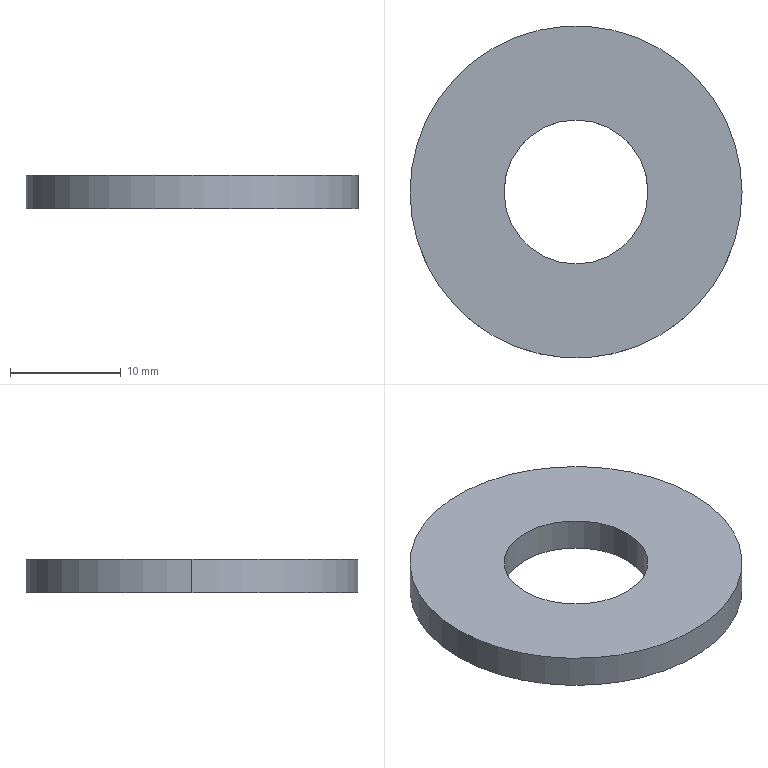Part | SolidWorks | features BaseBody 1 | 1 solid | 6 faces | box 30 x 30 x 3 mm | volume 1722 mm3 | cylinder 4 | plane 2 | commonest cylinder face diameters 13 x2 30 x2
STEP:
#1=CARTESIAN_POINT('',(-6.5,0.,-1.5));
#2=VERTEX_POINT('',#1);
#3=CARTESIAN_POINT('',(6.5,0.,-1.5));
#4=VERTEX_POINT('',#3);
#5=CARTESIAN_POINT('',(0.,0.,-1.5));
#6=DIRECTION('',(0.,0.,1.));
#7=DIRECTION('',(1.,0.,0.));
#8=AXIS2_PLACEMENT_3D('',#5,#6,#7);
#9=CIRCLE('',#8,6.5);
#10=EDGE_CURVE('',#2,#4,#9,.T.);
#11=ORIENTED_EDGE('',*,*,#10,.F.);
#12=CARTESIAN_POINT('',(-6.5,0.,1.5));
#13=VERTEX_POINT('',#12);
#14=CARTESIAN_POINT('',(-6.5,0.,0.));
#15=DIRECTION('',(0.,0.,1.));
#16=VECTOR('',#15,1000.);
#17=LINE('',#14,#16);
#18=EDGE_CURVE('',#2,#13,#17,.T.);
#19=ORIENTED_EDGE('',*,*,#18,.T.);
#20=CARTESIAN_POINT('',(6.5,0.,1.5));
#21=VERTEX_POINT('',#20);
#22=CARTESIAN_POINT('',(0.,0.,1.5));
#23=DIRECTION('',(0.,0.,-1.));
#24=DIRECTION('',(1.,0.,0.));
#25=AXIS2_PLACEMENT_3D('',#22,#23,#24);
#26=CIRCLE('',#25,6.5);
#27=EDGE_CURVE('',#21,#13,#26,.T.);
#28=ORIENTED_EDGE('',*,*,#27,.F.);
#29=CARTESIAN_POINT('',(6.5,0.,0.));
#30=DIRECTION('',(0.,0.,1.));
#31=VECTOR('',#30,1000.);
#32=LINE('',#29,#31);
#33=EDGE_CURVE('',#4,#21,#32,.T.);
#34=ORIENTED_EDGE('',*,*,#33,.F.);
#35=EDGE_LOOP('',(#11,#19,#28,#34));
#36=FACE_OUTER_BOUND('',#35,.T.);
#37=CARTESIAN_POINT('',(0.,0.,0.));
#38=DIRECTION('',(0.,0.,1.));
#39=DIRECTION('',(1.,0.,0.));
#40=AXIS2_PLACEMENT_3D('',#37,#38,#39);
#41=CYLINDRICAL_SURFACE('',#40,6.5);
#42=ADVANCED_FACE('',(#36),#41,.F.);
#43=CARTESIAN_POINT('',(15.,0.,-1.5));
#44=VERTEX_POINT('',#43);
#45=CARTESIAN_POINT('',(-15.,0.,-1.5));
#46=VERTEX_POINT('',#45);
#47=CARTESIAN_POINT('',(0.,0.,-1.5));
#48=DIRECTION('',(0.,0.,1.));
#49=DIRECTION('',(1.,0.,0.));
#50=AXIS2_PLACEMENT_3D('',#47,#48,#49);
#51=CIRCLE('',#50,15.);
#52=EDGE_CURVE('',#44,#46,#51,.T.);
#53=ORIENTED_EDGE('',*,*,#52,.T.);
#54=CARTESIAN_POINT('',(-15.,0.,1.5));
#55=VERTEX_POINT('',#54);
#56=CARTESIAN_POINT('',(-15.,0.,0.));
#57=DIRECTION('',(0.,0.,1.));
#58=VECTOR('',#57,1000.);
#59=LINE('',#56,#58);
#60=EDGE_CURVE('',#46,#55,#59,.T.);
#61=ORIENTED_EDGE('',*,*,#60,.T.);
#62=CARTESIAN_POINT('',(15.,0.,1.5));
#63=VERTEX_POINT('',#62);
#64=CARTESIAN_POINT('',(0.,0.,1.5));
#65=DIRECTION('',(0.,0.,1.));
#66=DIRECTION('',(1.,0.,0.));
#67=AXIS2_PLACEMENT_3D('',#64,#65,#66);
#68=CIRCLE('',#67,15.);
#69=EDGE_CURVE('',#63,#55,#68,.T.);
#70=ORIENTED_EDGE('',*,*,#69,.F.);
#71=CARTESIAN_POINT('',(15.,0.,0.));
#72=DIRECTION('',(0.,0.,1.));
#73=VECTOR('',#72,1000.);
#74=LINE('',#71,#73);
#75=EDGE_CURVE('',#44,#63,#74,.T.);
#76=ORIENTED_EDGE('',*,*,#75,.F.);
#77=EDGE_LOOP('',(#53,#61,#70,#76));
#78=FACE_OUTER_BOUND('',#77,.T.);
#79=CARTESIAN_POINT('',(0.,0.,0.));
#80=DIRECTION('',(0.,0.,1.));
#81=DIRECTION('',(1.,0.,0.));
#82=AXIS2_PLACEMENT_3D('',#79,#80,#81);
#83=CYLINDRICAL_SURFACE('',#82,15.);
#84=ADVANCED_FACE('',(#78),#83,.T.);
#85=ORIENTED_EDGE('',*,*,#27,.T.);
#86=CARTESIAN_POINT('',(0.,0.,1.5));
#87=DIRECTION('',(0.,0.,-1.));
#88=DIRECTION('',(1.,0.,0.));
#89=AXIS2_PLACEMENT_3D('',#86,#87,#88);
#90=CIRCLE('',#89,6.5);
#91=EDGE_CURVE('',#13,#21,#90,.T.);
#92=ORIENTED_EDGE('',*,*,#91,.T.);
#93=EDGE_LOOP('',(#85,#92));
#94=FACE_BOUND('',#93,.T.);
#95=ORIENTED_EDGE('',*,*,#69,.T.);
#96=CARTESIAN_POINT('',(0.,0.,1.5));
#97=DIRECTION('',(0.,0.,1.));
#98=DIRECTION('',(1.,0.,0.));
#99=AXIS2_PLACEMENT_3D('',#96,#97,#98);
#100=CIRCLE('',#99,15.);
#101=EDGE_CURVE('',#55,#63,#100,.T.);
#102=ORIENTED_EDGE('',*,*,#101,.T.);
#103=EDGE_LOOP('',(#95,#102));
#104=FACE_OUTER_BOUND('',#103,.T.);
#105=CARTESIAN_POINT('',(0.,0.,1.5));
#106=DIRECTION('',(0.,0.,1.));
#107=DIRECTION('',(1.,0.,0.));
#108=AXIS2_PLACEMENT_3D('',#105,#106,#107);
#109=PLANE('',#108);
#110=ADVANCED_FACE('',(#94,#104),#109,.T.);
#111=ORIENTED_EDGE('',*,*,#18,.F.);
#112=CARTESIAN_POINT('',(0.,0.,-1.5));
#113=DIRECTION('',(0.,0.,1.));
#114=DIRECTION('',(1.,0.,0.));
#115=AXIS2_PLACEMENT_3D('',#112,#113,#114);
#116=CIRCLE('',#115,6.5);
#117=EDGE_CURVE('',#4,#2,#116,.T.);
#118=ORIENTED_EDGE('',*,*,#117,.F.);
#119=ORIENTED_EDGE('',*,*,#33,.T.);
#120=ORIENTED_EDGE('',*,*,#91,.F.);
#121=EDGE_LOOP('',(#111,#118,#119,#120));
#122=FACE_OUTER_BOUND('',#121,.T.);
#123=CARTESIAN_POINT('',(0.,0.,0.));
#124=DIRECTION('',(0.,0.,1.));
#125=DIRECTION('',(1.,0.,0.));
#126=AXIS2_PLACEMENT_3D('',#123,#124,#125);
#127=CYLINDRICAL_SURFACE('',#126,6.5);
#128=ADVANCED_FACE('',(#122),#127,.F.);
#129=ORIENTED_EDGE('',*,*,#60,.F.);
#130=CARTESIAN_POINT('',(0.,0.,-1.5));
#131=DIRECTION('',(0.,0.,1.));
#132=DIRECTION('',(1.,0.,0.));
#133=AXIS2_PLACEMENT_3D('',#130,#131,#132);
#134=CIRCLE('',#133,15.);
#135=EDGE_CURVE('',#46,#44,#134,.T.);
#136=ORIENTED_EDGE('',*,*,#135,.T.);
#137=ORIENTED_EDGE('',*,*,#75,.T.);
#138=ORIENTED_EDGE('',*,*,#101,.F.);
#139=EDGE_LOOP('',(#129,#136,#137,#138));
#140=FACE_OUTER_BOUND('',#139,.T.);
#141=CARTESIAN_POINT('',(0.,0.,0.));
#142=DIRECTION('',(0.,0.,1.));
#143=DIRECTION('',(1.,0.,0.));
#144=AXIS2_PLACEMENT_3D('',#141,#142,#143);
#145=CYLINDRICAL_SURFACE('',#144,15.);
#146=ADVANCED_FACE('',(#140),#145,.T.);
#147=ORIENTED_EDGE('',*,*,#117,.T.);
#148=ORIENTED_EDGE('',*,*,#10,.T.);
#149=EDGE_LOOP('',(#147,#148));
#150=FACE_BOUND('',#149,.T.);
#151=ORIENTED_EDGE('',*,*,#52,.F.);
#152=ORIENTED_EDGE('',*,*,#135,.F.);
#153=EDGE_LOOP('',(#151,#152));
#154=FACE_OUTER_BOUND('',#153,.T.);
#155=CARTESIAN_POINT('',(0.,0.,-1.5));
#156=DIRECTION('',(0.,0.,1.));
#157=DIRECTION('',(1.,0.,0.));
#158=AXIS2_PLACEMENT_3D('',#155,#156,#157);
#159=PLANE('',#158);
#160=ADVANCED_FACE('',(#150,#154),#159,.F.);
#161=CLOSED_SHELL('',(#42,#84,#110,#128,#146,#160));
#162=MANIFOLD_SOLID_BREP('',#161);
#163=CARTESIAN_POINT('',(0.,0.,0.));
#164=DIRECTION('',(0.,0.,1.));
#165=DIRECTION('',(1.,0.,0.));
#166=AXIS2_PLACEMENT_3D('',#163,#164,#165);
#167=(LENGTH_UNIT()NAMED_UNIT(*)SI_UNIT(.MILLI.,.METRE.));
#168=UNCERTAINTY_MEASURE_WITH_UNIT(LENGTH_MEASURE(0.00001),#167,'','');
#169=(NAMED_UNIT(*)PLANE_ANGLE_UNIT()SI_UNIT($,.RADIAN.));
#170=(NAMED_UNIT(*)SI_UNIT($,.STERADIAN.)SOLID_ANGLE_UNIT());
#171=(GEOMETRIC_REPRESENTATION_CONTEXT(3)GLOBAL_UNCERTAINTY_ASSIGNED_CONTEXT((#168))GLOBAL_UNIT_ASSIGNED_CONTEXT((#167,#169,#170))REPRESENTATION_CONTEXT('',''));
#172=ADVANCED_BREP_SHAPE_REPRESENTATION('',(#162,#166),#171);